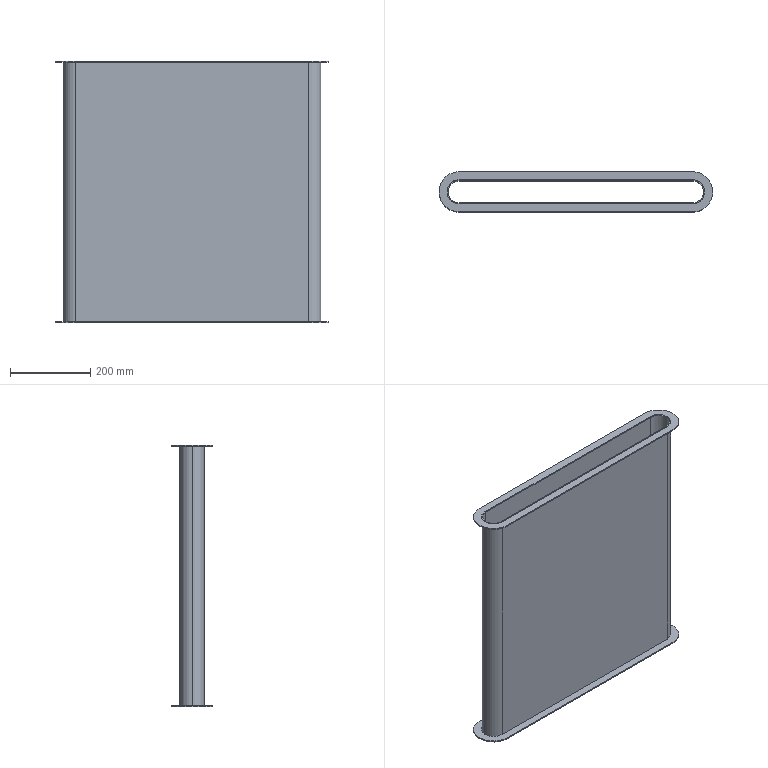Part | SolidWorks | features Extrusion 1, ICE 1, MirrorSolid 1 | 3 solids | 36 faces | box 680 x 100 x 650 mm | volume 2347902 mm3 | cylinder 18 | plane 18 | commonest cylinder face diameters 60 x9 100 x6 55 x3
STEP:
#1=CARTESIAN_POINT('',(0.,27.5,325.));
#2=VERTEX_POINT('',#1);
#3=CARTESIAN_POINT('',(-27.5,0.,325.));
#4=VERTEX_POINT('',#3);
#5=CARTESIAN_POINT('',(0.,0.,325.));
#6=DIRECTION('',(0.,0.,1.));
#7=DIRECTION('',(1.,0.,0.));
#8=AXIS2_PLACEMENT_3D('',#5,#6,#7);
#9=CIRCLE('',#8,27.5);
#10=EDGE_CURVE('',#2,#4,#9,.T.);
#11=ORIENTED_EDGE('',*,*,#10,.T.);
#12=CARTESIAN_POINT('',(-27.5,0.,-325.));
#13=VERTEX_POINT('',#12);
#14=CARTESIAN_POINT('',(-27.5,0.,325.));
#15=DIRECTION('',(0.,0.,-1.));
#16=VECTOR('',#15,1000.);
#17=LINE('',#14,#16);
#18=EDGE_CURVE('',#4,#13,#17,.T.);
#19=ORIENTED_EDGE('',*,*,#18,.T.);
#20=CARTESIAN_POINT('',(0.,27.5,-325.));
#21=VERTEX_POINT('',#20);
#22=CARTESIAN_POINT('',(0.,0.,-325.));
#23=DIRECTION('',(0.,0.,1.));
#24=DIRECTION('',(1.,0.,0.));
#25=AXIS2_PLACEMENT_3D('',#22,#23,#24);
#26=CIRCLE('',#25,27.5);
#27=EDGE_CURVE('',#21,#13,#26,.T.);
#28=ORIENTED_EDGE('',*,*,#27,.F.);
#29=CARTESIAN_POINT('',(0.,27.5,325.));
#30=DIRECTION('',(0.,0.,-1.));
#31=VECTOR('',#30,1000.);
#32=LINE('',#29,#31);
#33=EDGE_CURVE('',#2,#21,#32,.T.);
#34=ORIENTED_EDGE('',*,*,#33,.F.);
#35=EDGE_LOOP('',(#11,#19,#28,#34));
#36=FACE_OUTER_BOUND('',#35,.T.);
#37=CARTESIAN_POINT('',(0.,0.,325.));
#38=DIRECTION('',(0.,0.,-1.));
#39=DIRECTION('',(-1.,0.,0.));
#40=AXIS2_PLACEMENT_3D('',#37,#38,#39);
#41=CYLINDRICAL_SURFACE('',#40,27.5);
#42=ADVANCED_FACE('',(#36),#41,.F.);
#43=CARTESIAN_POINT('',(-30.,0.,325.));
#44=VERTEX_POINT('',#43);
#45=CARTESIAN_POINT('',(0.,-30.,325.));
#46=VERTEX_POINT('',#45);
#47=CARTESIAN_POINT('',(0.,0.,325.));
#48=DIRECTION('',(0.,0.,1.));
#49=DIRECTION('',(1.,0.,0.));
#50=AXIS2_PLACEMENT_3D('',#47,#48,#49);
#51=CIRCLE('',#50,30.);
#52=EDGE_CURVE('',#44,#46,#51,.T.);
#53=ORIENTED_EDGE('',*,*,#52,.F.);
#54=CARTESIAN_POINT('',(-30.,0.,-325.));
#55=VERTEX_POINT('',#54);
#56=CARTESIAN_POINT('',(-30.,0.,325.));
#57=DIRECTION('',(0.,0.,-1.));
#58=VECTOR('',#57,1000.);
#59=LINE('',#56,#58);
#60=EDGE_CURVE('',#44,#55,#59,.T.);
#61=ORIENTED_EDGE('',*,*,#60,.T.);
#62=CARTESIAN_POINT('',(0.,-30.,-325.));
#63=VERTEX_POINT('',#62);
#64=CARTESIAN_POINT('',(0.,0.,-325.));
#65=DIRECTION('',(0.,0.,1.));
#66=DIRECTION('',(1.,0.,0.));
#67=AXIS2_PLACEMENT_3D('',#64,#65,#66);
#68=CIRCLE('',#67,30.);
#69=EDGE_CURVE('',#55,#63,#68,.T.);
#70=ORIENTED_EDGE('',*,*,#69,.T.);
#71=CARTESIAN_POINT('',(0.,-30.,325.));
#72=DIRECTION('',(0.,0.,-1.));
#73=VECTOR('',#72,1000.);
#74=LINE('',#71,#73);
#75=EDGE_CURVE('',#46,#63,#74,.T.);
#76=ORIENTED_EDGE('',*,*,#75,.F.);
#77=EDGE_LOOP('',(#53,#61,#70,#76));
#78=FACE_OUTER_BOUND('',#77,.T.);
#79=CARTESIAN_POINT('',(0.,0.,325.));
#80=DIRECTION('',(0.,0.,-1.));
#81=DIRECTION('',(-1.,0.,0.));
#82=AXIS2_PLACEMENT_3D('',#79,#80,#81);
#83=CYLINDRICAL_SURFACE('',#82,30.);
#84=ADVANCED_FACE('',(#78),#83,.T.);
#85=CARTESIAN_POINT('',(0.,30.,325.));
#86=VERTEX_POINT('',#85);
#87=CARTESIAN_POINT('',(0.,0.,325.));
#88=DIRECTION('',(0.,0.,1.));
#89=DIRECTION('',(1.,0.,0.));
#90=AXIS2_PLACEMENT_3D('',#87,#88,#89);
#91=CIRCLE('',#90,30.);
#92=EDGE_CURVE('',#86,#44,#91,.T.);
#93=ORIENTED_EDGE('',*,*,#92,.T.);
#94=ORIENTED_EDGE('',*,*,#52,.T.);
#95=CARTESIAN_POINT('',(580.,-30.,325.));
#96=VERTEX_POINT('',#95);
#97=CARTESIAN_POINT('',(0.,-30.,325.));
#98=DIRECTION('',(1.,0.,0.));
#99=VECTOR('',#98,1000.);
#100=LINE('',#97,#99);
#101=EDGE_CURVE('',#46,#96,#100,.T.);
#102=ORIENTED_EDGE('',*,*,#101,.T.);
#103=CARTESIAN_POINT('',(580.,30.,325.));
#104=VERTEX_POINT('',#103);
#105=CARTESIAN_POINT('',(580.,0.,325.));
#106=DIRECTION('',(0.,0.,1.));
#107=DIRECTION('',(1.,0.,0.));
#108=AXIS2_PLACEMENT_3D('',#105,#106,#107);
#109=CIRCLE('',#108,30.);
#110=EDGE_CURVE('',#96,#104,#109,.T.);
#111=ORIENTED_EDGE('',*,*,#110,.T.);
#112=CARTESIAN_POINT('',(0.,30.,325.));
#113=DIRECTION('',(-1.,0.,0.));
#114=VECTOR('',#113,1000.);
#115=LINE('',#112,#114);
#116=EDGE_CURVE('',#104,#86,#115,.T.);
#117=ORIENTED_EDGE('',*,*,#116,.T.);
#118=EDGE_LOOP('',(#93,#94,#102,#111,#117));
#119=FACE_OUTER_BOUND('',#118,.T.);
#120=CARTESIAN_POINT('',(0.,-27.5,325.));
#121=VERTEX_POINT('',#120);
#122=CARTESIAN_POINT('',(580.,-27.5,325.));
#123=VERTEX_POINT('',#122);
#124=CARTESIAN_POINT('',(0.,-27.5,325.));
#125=DIRECTION('',(1.,0.,0.));
#126=VECTOR('',#125,1000.);
#127=LINE('',#124,#126);
#128=EDGE_CURVE('',#121,#123,#127,.T.);
#129=ORIENTED_EDGE('',*,*,#128,.F.);
#130=CARTESIAN_POINT('',(0.,0.,325.));
#131=DIRECTION('',(0.,0.,1.));
#132=DIRECTION('',(1.,0.,0.));
#133=AXIS2_PLACEMENT_3D('',#130,#131,#132);
#134=CIRCLE('',#133,27.5);
#135=EDGE_CURVE('',#4,#121,#134,.T.);
#136=ORIENTED_EDGE('',*,*,#135,.F.);
#137=ORIENTED_EDGE('',*,*,#10,.F.);
#138=CARTESIAN_POINT('',(580.,27.5,325.));
#139=VERTEX_POINT('',#138);
#140=CARTESIAN_POINT('',(0.,27.5,325.));
#141=DIRECTION('',(-1.,0.,0.));
#142=VECTOR('',#141,1000.);
#143=LINE('',#140,#142);
#144=EDGE_CURVE('',#139,#2,#143,.T.);
#145=ORIENTED_EDGE('',*,*,#144,.F.);
#146=CARTESIAN_POINT('',(580.,0.,325.));
#147=DIRECTION('',(0.,0.,1.));
#148=DIRECTION('',(1.,0.,0.));
#149=AXIS2_PLACEMENT_3D('',#146,#147,#148);
#150=CIRCLE('',#149,27.5);
#151=EDGE_CURVE('',#123,#139,#150,.T.);
#152=ORIENTED_EDGE('',*,*,#151,.F.);
#153=EDGE_LOOP('',(#129,#136,#137,#145,#152));
#154=FACE_BOUND('',#153,.T.);
#155=CARTESIAN_POINT('',(0.,0.,325.));
#156=DIRECTION('',(0.,0.,1.));
#157=DIRECTION('',(1.,0.,0.));
#158=AXIS2_PLACEMENT_3D('',#155,#156,#157);
#159=PLANE('',#158);
#160=ADVANCED_FACE('',(#119,#154),#159,.T.);
#161=CARTESIAN_POINT('',(0.,30.,-325.));
#162=VERTEX_POINT('',#161);
#163=CARTESIAN_POINT('',(0.,0.,-325.));
#164=DIRECTION('',(0.,0.,1.));
#165=DIRECTION('',(1.,0.,0.));
#166=AXIS2_PLACEMENT_3D('',#163,#164,#165);
#167=CIRCLE('',#166,30.);
#168=EDGE_CURVE('',#162,#55,#167,.T.);
#169=ORIENTED_EDGE('',*,*,#168,.F.);
#170=CARTESIAN_POINT('',(580.,30.,-325.));
#171=VERTEX_POINT('',#170);
#172=CARTESIAN_POINT('',(0.,30.,-325.));
#173=DIRECTION('',(-1.,0.,0.));
#174=VECTOR('',#173,1000.);
#175=LINE('',#172,#174);
#176=EDGE_CURVE('',#171,#162,#175,.T.);
#177=ORIENTED_EDGE('',*,*,#176,.F.);
#178=CARTESIAN_POINT('',(580.,-30.,-325.));
#179=VERTEX_POINT('',#178);
#180=CARTESIAN_POINT('',(580.,0.,-325.));
#181=DIRECTION('',(0.,0.,1.));
#182=DIRECTION('',(1.,0.,0.));
#183=AXIS2_PLACEMENT_3D('',#180,#181,#182);
#184=CIRCLE('',#183,30.);
#185=EDGE_CURVE('',#179,#171,#184,.T.);
#186=ORIENTED_EDGE('',*,*,#185,.F.);
#187=CARTESIAN_POINT('',(0.,-30.,-325.));
#188=DIRECTION('',(1.,0.,0.));
#189=VECTOR('',#188,1000.);
#190=LINE('',#187,#189);
#191=EDGE_CURVE('',#63,#179,#190,.T.);
#192=ORIENTED_EDGE('',*,*,#191,.F.);
#193=ORIENTED_EDGE('',*,*,#69,.F.);
#194=EDGE_LOOP('',(#169,#177,#186,#192,#193));
#195=FACE_OUTER_BOUND('',#194,.T.);
#196=ORIENTED_EDGE('',*,*,#27,.T.);
#197=CARTESIAN_POINT('',(0.,-27.5,-325.));
#198=VERTEX_POINT('',#197);
#199=CARTESIAN_POINT('',(0.,0.,-325.));
#200=DIRECTION('',(0.,0.,1.));
#201=DIRECTION('',(1.,0.,0.));
#202=AXIS2_PLACEMENT_3D('',#199,#200,#201);
#203=CIRCLE('',#202,27.5);
#204=EDGE_CURVE('',#13,#198,#203,.T.);
#205=ORIENTED_EDGE('',*,*,#204,.T.);
#206=CARTESIAN_POINT('',(580.,-27.5,-325.));
#207=VERTEX_POINT('',#206);
#208=CARTESIAN_POINT('',(0.,-27.5,-325.));
#209=DIRECTION('',(1.,0.,0.));
#210=VECTOR('',#209,1000.);
#211=LINE('',#208,#210);
#212=EDGE_CURVE('',#198,#207,#211,.T.);
#213=ORIENTED_EDGE('',*,*,#212,.T.);
#214=CARTESIAN_POINT('',(580.,27.5,-325.));
#215=VERTEX_POINT('',#214);
#216=CARTESIAN_POINT('',(580.,0.,-325.));
#217=DIRECTION('',(0.,0.,1.));
#218=DIRECTION('',(1.,0.,0.));
#219=AXIS2_PLACEMENT_3D('',#216,#217,#218);
#220=CIRCLE('',#219,27.5);
#221=EDGE_CURVE('',#207,#215,#220,.T.);
#222=ORIENTED_EDGE('',*,*,#221,.T.);
#223=CARTESIAN_POINT('',(0.,27.5,-325.));
#224=DIRECTION('',(-1.,0.,0.));
#225=VECTOR('',#224,1000.);
#226=LINE('',#223,#225);
#227=EDGE_CURVE('',#215,#21,#226,.T.);
#228=ORIENTED_EDGE('',*,*,#227,.T.);
#229=EDGE_LOOP('',(#196,#205,#213,#222,#228));
#230=FACE_BOUND('',#229,.T.);
#231=CARTESIAN_POINT('',(0.,0.,-325.));
#232=DIRECTION('',(0.,0.,1.));
#233=DIRECTION('',(1.,0.,0.));
#234=AXIS2_PLACEMENT_3D('',#231,#232,#233);
#235=PLANE('',#234);
#236=ADVANCED_FACE('',(#195,#230),#235,.F.);
#237=ORIENTED_EDGE('',*,*,#60,.F.);
#238=ORIENTED_EDGE('',*,*,#92,.F.);
#239=CARTESIAN_POINT('',(0.,30.,325.));
#240=DIRECTION('',(0.,0.,-1.));
#241=VECTOR('',#240,1000.);
#242=LINE('',#239,#241);
#243=EDGE_CURVE('',#86,#162,#242,.T.);
#244=ORIENTED_EDGE('',*,*,#243,.T.);
#245=ORIENTED_EDGE('',*,*,#168,.T.);
#246=EDGE_LOOP('',(#237,#238,#244,#245));
#247=FACE_OUTER_BOUND('',#246,.T.);
#248=CARTESIAN_POINT('',(0.,0.,325.));
#249=DIRECTION('',(0.,0.,-1.));
#250=DIRECTION('',(-1.,0.,0.));
#251=AXIS2_PLACEMENT_3D('',#248,#249,#250);
#252=CYLINDRICAL_SURFACE('',#251,30.);
#253=ADVANCED_FACE('',(#247),#252,.T.);
#254=ORIENTED_EDGE('',*,*,#191,.T.);
#255=CARTESIAN_POINT('',(580.,-30.,325.));
#256=DIRECTION('',(0.,0.,-1.));
#257=VECTOR('',#256,1000.);
#258=LINE('',#255,#257);
#259=EDGE_CURVE('',#96,#179,#258,.T.);
#260=ORIENTED_EDGE('',*,*,#259,.F.);
#261=ORIENTED_EDGE('',*,*,#101,.F.);
#262=ORIENTED_EDGE('',*,*,#75,.T.);
#263=EDGE_LOOP('',(#254,#260,#261,#262));
#264=FACE_OUTER_BOUND('',#263,.T.);
#265=CARTESIAN_POINT('',(0.,-30.,325.));
#266=DIRECTION('',(0.,1.,0.));
#267=DIRECTION('',(0.,0.,1.));
#268=AXIS2_PLACEMENT_3D('',#265,#266,#267);
#269=PLANE('',#268);
#270=ADVANCED_FACE('',(#264),#269,.F.);
#271=ORIENTED_EDGE('',*,*,#185,.T.);
#272=CARTESIAN_POINT('',(580.,30.,325.));
#273=DIRECTION('',(0.,0.,-1.));
#274=VECTOR('',#273,1000.);
#275=LINE('',#272,#274);
#276=EDGE_CURVE('',#104,#171,#275,.T.);
#277=ORIENTED_EDGE('',*,*,#276,.F.);
#278=ORIENTED_EDGE('',*,*,#110,.F.);
#279=ORIENTED_EDGE('',*,*,#259,.T.);
#280=EDGE_LOOP('',(#271,#277,#278,#279));
#281=FACE_OUTER_BOUND('',#280,.T.);
#282=CARTESIAN_POINT('',(580.,0.,325.));
#283=DIRECTION('',(0.,0.,-1.));
#284=DIRECTION('',(-1.,0.,0.));
#285=AXIS2_PLACEMENT_3D('',#282,#283,#284);
#286=CYLINDRICAL_SURFACE('',#285,30.);
#287=ADVANCED_FACE('',(#281),#286,.T.);
#288=ORIENTED_EDGE('',*,*,#176,.T.);
#289=ORIENTED_EDGE('',*,*,#243,.F.);
#290=ORIENTED_EDGE('',*,*,#116,.F.);
#291=ORIENTED_EDGE('',*,*,#276,.T.);
#292=EDGE_LOOP('',(#288,#289,#290,#291));
#293=FACE_OUTER_BOUND('',#292,.T.);
#294=CARTESIAN_POINT('',(0.,30.,325.));
#295=DIRECTION('',(0.,-1.,0.));
#296=DIRECTION('',(0.,0.,-1.));
#297=AXIS2_PLACEMENT_3D('',#294,#295,#296);
#298=PLANE('',#297);
#299=ADVANCED_FACE('',(#293),#298,.F.);
#300=ORIENTED_EDGE('',*,*,#18,.F.);
#301=ORIENTED_EDGE('',*,*,#135,.T.);
#302=CARTESIAN_POINT('',(0.,-27.5,325.));
#303=DIRECTION('',(0.,0.,-1.));
#304=VECTOR('',#303,1000.);
#305=LINE('',#302,#304);
#306=EDGE_CURVE('',#121,#198,#305,.T.);
#307=ORIENTED_EDGE('',*,*,#306,.T.);
#308=ORIENTED_EDGE('',*,*,#204,.F.);
#309=EDGE_LOOP('',(#300,#301,#307,#308));
#310=FACE_OUTER_BOUND('',#309,.T.);
#311=CARTESIAN_POINT('',(0.,0.,325.));
#312=DIRECTION('',(0.,0.,-1.));
#313=DIRECTION('',(-1.,0.,0.));
#314=AXIS2_PLACEMENT_3D('',#311,#312,#313);
#315=CYLINDRICAL_SURFACE('',#314,27.5);
#316=ADVANCED_FACE('',(#310),#315,.F.);
#317=ORIENTED_EDGE('',*,*,#212,.F.);
#318=ORIENTED_EDGE('',*,*,#306,.F.);
#319=ORIENTED_EDGE('',*,*,#128,.T.);
#320=CARTESIAN_POINT('',(580.,-27.5,325.));
#321=DIRECTION('',(0.,0.,-1.));
#322=VECTOR('',#321,1000.);
#323=LINE('',#320,#322);
#324=EDGE_CURVE('',#123,#207,#323,.T.);
#325=ORIENTED_EDGE('',*,*,#324,.T.);
#326=EDGE_LOOP('',(#317,#318,#319,#325));
#327=FACE_OUTER_BOUND('',#326,.T.);
#328=CARTESIAN_POINT('',(0.,-27.5,325.));
#329=DIRECTION('',(0.,1.,0.));
#330=DIRECTION('',(0.,0.,1.));
#331=AXIS2_PLACEMENT_3D('',#328,#329,#330);
#332=PLANE('',#331);
#333=ADVANCED_FACE('',(#327),#332,.T.);
#334=ORIENTED_EDGE('',*,*,#221,.F.);
#335=ORIENTED_EDGE('',*,*,#324,.F.);
#336=ORIENTED_EDGE('',*,*,#151,.T.);
#337=CARTESIAN_POINT('',(580.,27.5,325.));
#338=DIRECTION('',(0.,0.,-1.));
#339=VECTOR('',#338,1000.);
#340=LINE('',#337,#339);
#341=EDGE_CURVE('',#139,#215,#340,.T.);
#342=ORIENTED_EDGE('',*,*,#341,.T.);
#343=EDGE_LOOP('',(#334,#335,#336,#342));
#344=FACE_OUTER_BOUND('',#343,.T.);
#345=CARTESIAN_POINT('',(580.,0.,325.));
#346=DIRECTION('',(0.,0.,-1.));
#347=DIRECTION('',(-1.,0.,0.));
#348=AXIS2_PLACEMENT_3D('',#345,#346,#347);
#349=CYLINDRICAL_SURFACE('',#348,27.5);
#350=ADVANCED_FACE('',(#344),#349,.F.);
#351=ORIENTED_EDGE('',*,*,#227,.F.);
#352=ORIENTED_EDGE('',*,*,#341,.F.);
#353=ORIENTED_EDGE('',*,*,#144,.T.);
#354=ORIENTED_EDGE('',*,*,#33,.T.);
#355=EDGE_LOOP('',(#351,#352,#353,#354));
#356=FACE_OUTER_BOUND('',#355,.T.);
#357=CARTESIAN_POINT('',(0.,27.5,325.));
#358=DIRECTION('',(0.,-1.,0.));
#359=DIRECTION('',(0.,0.,-1.));
#360=AXIS2_PLACEMENT_3D('',#357,#358,#359);
#361=PLANE('',#360);
#362=ADVANCED_FACE('',(#356),#361,.T.);
#363=CLOSED_SHELL('',(#42,#84,#160,#236,#253,#270,#287,#299,#316,#333,#350,#362));
#364=MANIFOLD_SOLID_BREP('',#363);
#365=CARTESIAN_POINT('',(610.,0.,322.));
#366=VERTEX_POINT('',#365);
#367=CARTESIAN_POINT('',(580.,30.,322.));
#368=VERTEX_POINT('',#367);
#369=CARTESIAN_POINT('',(580.,0.,322.));
#370=DIRECTION('',(0.,0.,1.));
#371=DIRECTION('',(1.,0.,0.));
#372=AXIS2_PLACEMENT_3D('',#369,#370,#371);
#373=CIRCLE('',#372,30.);
#374=EDGE_CURVE('',#366,#368,#373,.T.);
#375=ORIENTED_EDGE('',*,*,#374,.F.);
#376=CARTESIAN_POINT('',(610.,0.,325.));
#377=VERTEX_POINT('',#376);
#378=CARTESIAN_POINT('',(610.,0.,322.));
#379=DIRECTION('',(0.,0.,1.));
#380=VECTOR('',#379,1000.);
#381=LINE('',#378,#380);
#382=EDGE_CURVE('',#366,#377,#381,.T.);
#383=ORIENTED_EDGE('',*,*,#382,.T.);
#384=CARTESIAN_POINT('',(580.,30.,325.));
#385=VERTEX_POINT('',#384);
#386=CARTESIAN_POINT('',(580.,0.,325.));
#387=DIRECTION('',(0.,0.,1.));
#388=DIRECTION('',(1.,0.,0.));
#389=AXIS2_PLACEMENT_3D('',#386,#387,#388);
#390=CIRCLE('',#389,30.);
#391=EDGE_CURVE('',#377,#385,#390,.T.);
#392=ORIENTED_EDGE('',*,*,#391,.T.);
#393=CARTESIAN_POINT('',(580.,30.,322.));
#394=DIRECTION('',(0.,0.,1.));
#395=VECTOR('',#394,1000.);
#396=LINE('',#393,#395);
#397=EDGE_CURVE('',#368,#385,#396,.T.);
#398=ORIENTED_EDGE('',*,*,#397,.F.);
#399=EDGE_LOOP('',(#375,#383,#392,#398));
#400=FACE_OUTER_BOUND('',#399,.T.);
#401=CARTESIAN_POINT('',(580.,0.,322.));
#402=DIRECTION('',(0.,0.,1.));
#403=DIRECTION('',(1.,0.,0.));
#404=AXIS2_PLACEMENT_3D('',#401,#402,#403);
#405=CYLINDRICAL_SURFACE('',#404,30.);
#406=ADVANCED_FACE('',(#400),#405,.F.);
#407=CARTESIAN_POINT('',(580.,-50.,322.));
#408=VERTEX_POINT('',#407);
#409=CARTESIAN_POINT('',(630.,0.,322.));
#410=VERTEX_POINT('',#409);
#411=CARTESIAN_POINT('',(580.,0.,322.));
#412=DIRECTION('',(0.,0.,1.));
#413=DIRECTION('',(1.,0.,0.));
#414=AXIS2_PLACEMENT_3D('',#411,#412,#413);
#415=CIRCLE('',#414,50.);
#416=EDGE_CURVE('',#408,#410,#415,.T.);
#417=ORIENTED_EDGE('',*,*,#416,.T.);
#418=CARTESIAN_POINT('',(630.,0.,325.));
#419=VERTEX_POINT('',#418);
#420=CARTESIAN_POINT('',(630.,0.,322.));
#421=DIRECTION('',(0.,0.,1.));
#422=VECTOR('',#421,1000.);
#423=LINE('',#420,#422);
#424=EDGE_CURVE('',#410,#419,#423,.T.);
#425=ORIENTED_EDGE('',*,*,#424,.T.);
#426=CARTESIAN_POINT('',(580.,-50.,325.));
#427=VERTEX_POINT('',#426);
#428=CARTESIAN_POINT('',(580.,0.,325.));
#429=DIRECTION('',(0.,0.,1.));
#430=DIRECTION('',(1.,0.,0.));
#431=AXIS2_PLACEMENT_3D('',#428,#429,#430);
#432=CIRCLE('',#431,50.);
#433=EDGE_CURVE('',#427,#419,#432,.T.);
#434=ORIENTED_EDGE('',*,*,#433,.F.);
#435=CARTESIAN_POINT('',(580.,-50.,322.));
#436=DIRECTION('',(0.,0.,1.));
#437=VECTOR('',#436,1000.);
#438=LINE('',#435,#437);
#439=EDGE_CURVE('',#408,#427,#438,.T.);
#440=ORIENTED_EDGE('',*,*,#439,.F.);
#441=EDGE_LOOP('',(#417,#425,#434,#440));
#442=FACE_OUTER_BOUND('',#441,.T.);
#443=CARTESIAN_POINT('',(580.,0.,322.));
#444=DIRECTION('',(0.,0.,1.));
#445=DIRECTION('',(1.,0.,0.));
#446=AXIS2_PLACEMENT_3D('',#443,#444,#445);
#447=CYLINDRICAL_SURFACE('',#446,50.);
#448=ADVANCED_FACE('',(#442),#447,.T.);
#449=ORIENTED_EDGE('',*,*,#424,.F.);
#450=CARTESIAN_POINT('',(580.,50.,322.));
#451=VERTEX_POINT('',#450);
#452=CARTESIAN_POINT('',(580.,0.,322.));
#453=DIRECTION('',(0.,0.,1.));
#454=DIRECTION('',(1.,0.,0.));
#455=AXIS2_PLACEMENT_3D('',#452,#453,#454);
#456=CIRCLE('',#455,50.);
#457=EDGE_CURVE('',#410,#451,#456,.T.);
#458=ORIENTED_EDGE('',*,*,#457,.T.);
#459=CARTESIAN_POINT('',(580.,50.,325.));
#460=VERTEX_POINT('',#459);
#461=CARTESIAN_POINT('',(580.,50.,322.));
#462=DIRECTION('',(0.,0.,1.));
#463=VECTOR('',#462,1000.);
#464=LINE('',#461,#463);
#465=EDGE_CURVE('',#451,#460,#464,.T.);
#466=ORIENTED_EDGE('',*,*,#465,.T.);
#467=CARTESIAN_POINT('',(580.,0.,325.));
#468=DIRECTION('',(0.,0.,1.));
#469=DIRECTION('',(1.,0.,0.));
#470=AXIS2_PLACEMENT_3D('',#467,#468,#469);
#471=CIRCLE('',#470,50.);
#472=EDGE_CURVE('',#419,#460,#471,.T.);
#473=ORIENTED_EDGE('',*,*,#472,.F.);
#474=EDGE_LOOP('',(#449,#458,#466,#473));
#475=FACE_OUTER_BOUND('',#474,.T.);
#476=CARTESIAN_POINT('',(580.,0.,322.));
#477=DIRECTION('',(0.,0.,1.));
#478=DIRECTION('',(1.,0.,0.));
#479=AXIS2_PLACEMENT_3D('',#476,#477,#478);
#480=CYLINDRICAL_SURFACE('',#479,50.);
#481=ADVANCED_FACE('',(#475),#480,.T.);
#482=CARTESIAN_POINT('',(0.,-50.,325.));
#483=VERTEX_POINT('',#482);
#484=CARTESIAN_POINT('',(0.,-50.,325.));
#485=DIRECTION('',(1.,0.,0.));
#486=VECTOR('',#485,1000.);
#487=LINE('',#484,#486);
#488=EDGE_CURVE('',#483,#427,#487,.T.);
#489=ORIENTED_EDGE('',*,*,#488,.F.);
#490=CARTESIAN_POINT('',(0.,-50.,322.));
#491=VERTEX_POINT('',#490);
#492=CARTESIAN_POINT('',(0.,-50.,322.));
#493=DIRECTION('',(0.,0.,1.));
#494=VECTOR('',#493,1000.);
#495=LINE('',#492,#494);
#496=EDGE_CURVE('',#491,#483,#495,.T.);
#497=ORIENTED_EDGE('',*,*,#496,.F.);
#498=CARTESIAN_POINT('',(0.,-50.,322.));
#499=DIRECTION('',(1.,0.,0.));
#500=VECTOR('',#499,1000.);
#501=LINE('',#498,#500);
#502=EDGE_CURVE('',#491,#408,#501,.T.);
#503=ORIENTED_EDGE('',*,*,#502,.T.);
#504=ORIENTED_EDGE('',*,*,#439,.T.);
#505=EDGE_LOOP('',(#489,#497,#503,#504));
#506=FACE_OUTER_BOUND('',#505,.T.);
#507=CARTESIAN_POINT('',(0.,-50.,322.));
#508=DIRECTION('',(0.,-1.,0.));
#509=DIRECTION('',(1.,0.,0.));
#510=AXIS2_PLACEMENT_3D('',#507,#508,#509);
#511=PLANE('',#510);
#512=ADVANCED_FACE('',(#506),#511,.T.);
#513=CARTESIAN_POINT('',(0.,50.,325.));
#514=VERTEX_POINT('',#513);
#515=CARTESIAN_POINT('',(0.,0.,325.));
#516=DIRECTION('',(0.,0.,1.));
#517=DIRECTION('',(1.,0.,0.));
#518=AXIS2_PLACEMENT_3D('',#515,#516,#517);
#519=CIRCLE('',#518,50.);
#520=EDGE_CURVE('',#514,#483,#519,.T.);
#521=ORIENTED_EDGE('',*,*,#520,.F.);
#522=CARTESIAN_POINT('',(0.,50.,322.));
#523=VERTEX_POINT('',#522);
#524=CARTESIAN_POINT('',(0.,50.,322.));
#525=DIRECTION('',(0.,0.,1.));
#526=VECTOR('',#525,1000.);
#527=LINE('',#524,#526);
#528=EDGE_CURVE('',#523,#514,#527,.T.);
#529=ORIENTED_EDGE('',*,*,#528,.F.);
#530=CARTESIAN_POINT('',(0.,0.,322.));
#531=DIRECTION('',(0.,0.,1.));
#532=DIRECTION('',(1.,0.,0.));
#533=AXIS2_PLACEMENT_3D('',#530,#531,#532);
#534=CIRCLE('',#533,50.);
#535=EDGE_CURVE('',#523,#491,#534,.T.);
#536=ORIENTED_EDGE('',*,*,#535,.T.);
#537=ORIENTED_EDGE('',*,*,#496,.T.);
#538=EDGE_LOOP('',(#521,#529,#536,#537));
#539=FACE_OUTER_BOUND('',#538,.T.);
#540=CARTESIAN_POINT('',(0.,0.,322.));
#541=DIRECTION('',(0.,0.,1.));
#542=DIRECTION('',(1.,0.,0.));
#543=AXIS2_PLACEMENT_3D('',#540,#541,#542);
#544=CYLINDRICAL_SURFACE('',#543,50.);
#545=ADVANCED_FACE('',(#539),#544,.T.);
#546=CARTESIAN_POINT('',(580.,50.,325.));
#547=DIRECTION('',(-1.,0.,0.));
#548=VECTOR('',#547,1000.);
#549=LINE('',#546,#548);
#550=EDGE_CURVE('',#460,#514,#549,.T.);
#551=ORIENTED_EDGE('',*,*,#550,.F.);
#552=ORIENTED_EDGE('',*,*,#465,.F.);
#553=CARTESIAN_POINT('',(580.,50.,322.));
#554=DIRECTION('',(-1.,0.,0.));
#555=VECTOR('',#554,1000.);
#556=LINE('',#553,#555);
#557=EDGE_CURVE('',#451,#523,#556,.T.);
#558=ORIENTED_EDGE('',*,*,#557,.T.);
#559=ORIENTED_EDGE('',*,*,#528,.T.);
#560=EDGE_LOOP('',(#551,#552,#558,#559));
#561=FACE_OUTER_BOUND('',#560,.T.);
#562=CARTESIAN_POINT('',(580.,50.,322.));
#563=DIRECTION('',(0.,1.,0.));
#564=DIRECTION('',(-1.,0.,0.));
#565=AXIS2_PLACEMENT_3D('',#562,#563,#564);
#566=PLANE('',#565);
#567=ADVANCED_FACE('',(#561),#566,.T.);
#568=CARTESIAN_POINT('',(0.,30.,322.));
#569=VERTEX_POINT('',#568);
#570=CARTESIAN_POINT('',(580.,30.,322.));
#571=DIRECTION('',(-1.,0.,0.));
#572=VECTOR('',#571,1000.);
#573=LINE('',#570,#572);
#574=EDGE_CURVE('',#368,#569,#573,.T.);
#575=ORIENTED_EDGE('',*,*,#574,.T.);
#576=CARTESIAN_POINT('',(0.,-30.,322.));
#577=VERTEX_POINT('',#576);
#578=CARTESIAN_POINT('',(0.,0.,322.));
#579=DIRECTION('',(0.,0.,1.));
#580=DIRECTION('',(1.,0.,0.));
#581=AXIS2_PLACEMENT_3D('',#578,#579,#580);
#582=CIRCLE('',#581,30.);
#583=EDGE_CURVE('',#569,#577,#582,.T.);
#584=ORIENTED_EDGE('',*,*,#583,.T.);
#585=CARTESIAN_POINT('',(580.,-30.,322.));
#586=VERTEX_POINT('',#585);
#587=CARTESIAN_POINT('',(0.,-30.,322.));
#588=DIRECTION('',(1.,0.,0.));
#589=VECTOR('',#588,1000.);
#590=LINE('',#587,#589);
#591=EDGE_CURVE('',#577,#586,#590,.T.);
#592=ORIENTED_EDGE('',*,*,#591,.T.);
#593=CARTESIAN_POINT('',(580.,0.,322.));
#594=DIRECTION('',(0.,0.,1.));
#595=DIRECTION('',(1.,0.,0.));
#596=AXIS2_PLACEMENT_3D('',#593,#594,#595);
#597=CIRCLE('',#596,30.);
#598=EDGE_CURVE('',#586,#366,#597,.T.);
#599=ORIENTED_EDGE('',*,*,#598,.T.);
#600=ORIENTED_EDGE('',*,*,#374,.T.);
#601=EDGE_LOOP('',(#575,#584,#592,#599,#600));
#602=FACE_BOUND('',#601,.T.);
#603=ORIENTED_EDGE('',*,*,#416,.F.);
#604=ORIENTED_EDGE('',*,*,#502,.F.);
#605=ORIENTED_EDGE('',*,*,#535,.F.);
#606=ORIENTED_EDGE('',*,*,#557,.F.);
#607=ORIENTED_EDGE('',*,*,#457,.F.);
#608=EDGE_LOOP('',(#603,#604,#605,#606,#607));
#609=FACE_OUTER_BOUND('',#608,.T.);
#610=CARTESIAN_POINT('',(580.,0.,322.));
#611=DIRECTION('',(0.,0.,1.));
#612=DIRECTION('',(1.,0.,0.));
#613=AXIS2_PLACEMENT_3D('',#610,#611,#612);
#614=PLANE('',#613);
#615=ADVANCED_FACE('',(#602,#609),#614,.F.);
#616=CARTESIAN_POINT('',(0.,30.,325.));
#617=VERTEX_POINT('',#616);
#618=CARTESIAN_POINT('',(0.,-30.,325.));
#619=VERTEX_POINT('',#618);
#620=CARTESIAN_POINT('',(0.,0.,325.));
#621=DIRECTION('',(0.,0.,1.));
#622=DIRECTION('',(1.,0.,0.));
#623=AXIS2_PLACEMENT_3D('',#620,#621,#622);
#624=CIRCLE('',#623,30.);
#625=EDGE_CURVE('',#617,#619,#624,.T.);
#626=ORIENTED_EDGE('',*,*,#625,.F.);
#627=CARTESIAN_POINT('',(580.,30.,325.));
#628=DIRECTION('',(-1.,0.,0.));
#629=VECTOR('',#628,1000.);
#630=LINE('',#627,#629);
#631=EDGE_CURVE('',#385,#617,#630,.T.);
#632=ORIENTED_EDGE('',*,*,#631,.F.);
#633=ORIENTED_EDGE('',*,*,#391,.F.);
#634=CARTESIAN_POINT('',(580.,-30.,325.));
#635=VERTEX_POINT('',#634);
#636=CARTESIAN_POINT('',(580.,0.,325.));
#637=DIRECTION('',(0.,0.,1.));
#638=DIRECTION('',(1.,0.,0.));
#639=AXIS2_PLACEMENT_3D('',#636,#637,#638);
#640=CIRCLE('',#639,30.);
#641=EDGE_CURVE('',#635,#377,#640,.T.);
#642=ORIENTED_EDGE('',*,*,#641,.F.);
#643=CARTESIAN_POINT('',(0.,-30.,325.));
#644=DIRECTION('',(1.,0.,0.));
#645=VECTOR('',#644,1000.);
#646=LINE('',#643,#645);
#647=EDGE_CURVE('',#619,#635,#646,.T.);
#648=ORIENTED_EDGE('',*,*,#647,.F.);
#649=EDGE_LOOP('',(#626,#632,#633,#642,#648));
#650=FACE_BOUND('',#649,.T.);
#651=ORIENTED_EDGE('',*,*,#433,.T.);
#652=ORIENTED_EDGE('',*,*,#472,.T.);
#653=ORIENTED_EDGE('',*,*,#550,.T.);
#654=ORIENTED_EDGE('',*,*,#520,.T.);
#655=ORIENTED_EDGE('',*,*,#488,.T.);
#656=EDGE_LOOP('',(#651,#652,#653,#654,#655));
#657=FACE_OUTER_BOUND('',#656,.T.);
#658=CARTESIAN_POINT('',(580.,0.,325.));
#659=DIRECTION('',(0.,0.,1.));
#660=DIRECTION('',(1.,0.,0.));
#661=AXIS2_PLACEMENT_3D('',#658,#659,#660);
#662=PLANE('',#661);
#663=ADVANCED_FACE('',(#650,#657),#662,.T.);
#664=ORIENTED_EDGE('',*,*,#625,.T.);
#665=CARTESIAN_POINT('',(0.,-30.,322.));
#666=DIRECTION('',(0.,0.,1.));
#667=VECTOR('',#666,1000.);
#668=LINE('',#665,#667);
#669=EDGE_CURVE('',#577,#619,#668,.T.);
#670=ORIENTED_EDGE('',*,*,#669,.F.);
#671=ORIENTED_EDGE('',*,*,#583,.F.);
#672=CARTESIAN_POINT('',(0.,30.,322.));
#673=DIRECTION('',(0.,0.,1.));
#674=VECTOR('',#673,1000.);
#675=LINE('',#672,#674);
#676=EDGE_CURVE('',#569,#617,#675,.T.);
#677=ORIENTED_EDGE('',*,*,#676,.T.);
#678=EDGE_LOOP('',(#664,#670,#671,#677));
#679=FACE_OUTER_BOUND('',#678,.T.);
#680=CARTESIAN_POINT('',(0.,0.,322.));
#681=DIRECTION('',(0.,0.,1.));
#682=DIRECTION('',(1.,0.,0.));
#683=AXIS2_PLACEMENT_3D('',#680,#681,#682);
#684=CYLINDRICAL_SURFACE('',#683,30.);
#685=ADVANCED_FACE('',(#679),#684,.F.);
#686=ORIENTED_EDGE('',*,*,#631,.T.);
#687=ORIENTED_EDGE('',*,*,#676,.F.);
#688=ORIENTED_EDGE('',*,*,#574,.F.);
#689=ORIENTED_EDGE('',*,*,#397,.T.);
#690=EDGE_LOOP('',(#686,#687,#688,#689));
#691=FACE_OUTER_BOUND('',#690,.T.);
#692=CARTESIAN_POINT('',(580.,30.,322.));
#693=DIRECTION('',(0.,1.,0.));
#694=DIRECTION('',(0.,0.,1.));
#695=AXIS2_PLACEMENT_3D('',#692,#693,#694);
#696=PLANE('',#695);
#697=ADVANCED_FACE('',(#691),#696,.F.);
#698=ORIENTED_EDGE('',*,*,#382,.F.);
#699=ORIENTED_EDGE('',*,*,#598,.F.);
#700=CARTESIAN_POINT('',(580.,-30.,322.));
#701=DIRECTION('',(0.,0.,1.));
#702=VECTOR('',#701,1000.);
#703=LINE('',#700,#702);
#704=EDGE_CURVE('',#586,#635,#703,.T.);
#705=ORIENTED_EDGE('',*,*,#704,.T.);
#706=ORIENTED_EDGE('',*,*,#641,.T.);
#707=EDGE_LOOP('',(#698,#699,#705,#706));
#708=FACE_OUTER_BOUND('',#707,.T.);
#709=CARTESIAN_POINT('',(580.,0.,322.));
#710=DIRECTION('',(0.,0.,1.));
#711=DIRECTION('',(1.,0.,0.));
#712=AXIS2_PLACEMENT_3D('',#709,#710,#711);
#713=CYLINDRICAL_SURFACE('',#712,30.);
#714=ADVANCED_FACE('',(#708),#713,.F.);
#715=ORIENTED_EDGE('',*,*,#647,.T.);
#716=ORIENTED_EDGE('',*,*,#704,.F.);
#717=ORIENTED_EDGE('',*,*,#591,.F.);
#718=ORIENTED_EDGE('',*,*,#669,.T.);
#719=EDGE_LOOP('',(#715,#716,#717,#718));
#720=FACE_OUTER_BOUND('',#719,.T.);
#721=CARTESIAN_POINT('',(0.,-30.,322.));
#722=DIRECTION('',(0.,-1.,0.));
#723=DIRECTION('',(0.,0.,-1.));
#724=AXIS2_PLACEMENT_3D('',#721,#722,#723);
#725=PLANE('',#724);
#726=ADVANCED_FACE('',(#720),#725,.F.);
#727=CLOSED_SHELL('',(#406,#448,#481,#512,#545,#567,#615,#663,#685,#697,#714,#726));
#728=MANIFOLD_SOLID_BREP('',#727);
#729=CARTESIAN_POINT('',(580.,-30.,-322.));
#730=VERTEX_POINT('',#729);
#731=CARTESIAN_POINT('',(610.,0.,-322.));
#732=VERTEX_POINT('',#731);
#733=CARTESIAN_POINT('',(580.,0.,-322.));
#734=DIRECTION('',(0.,0.,1.));
#735=DIRECTION('',(1.,0.,0.));
#736=AXIS2_PLACEMENT_3D('',#733,#734,#735);
#737=CIRCLE('',#736,30.);
#738=EDGE_CURVE('',#730,#732,#737,.T.);
#739=ORIENTED_EDGE('',*,*,#738,.T.);
#740=CARTESIAN_POINT('',(610.,0.,-325.));
#741=VERTEX_POINT('',#740);
#742=CARTESIAN_POINT('',(610.,0.,-322.));
#743=DIRECTION('',(0.,0.,-1.));
#744=VECTOR('',#743,1000.);
#745=LINE('',#742,#744);
#746=EDGE_CURVE('',#732,#741,#745,.T.);
#747=ORIENTED_EDGE('',*,*,#746,.T.);
#748=CARTESIAN_POINT('',(580.,-30.,-325.));
#749=VERTEX_POINT('',#748);
#750=CARTESIAN_POINT('',(580.,0.,-325.));
#751=DIRECTION('',(0.,0.,1.));
#752=DIRECTION('',(1.,0.,0.));
#753=AXIS2_PLACEMENT_3D('',#750,#751,#752);
#754=CIRCLE('',#753,30.);
#755=EDGE_CURVE('',#749,#741,#754,.T.);
#756=ORIENTED_EDGE('',*,*,#755,.F.);
#757=CARTESIAN_POINT('',(580.,-30.,-322.));
#758=DIRECTION('',(0.,0.,-1.));
#759=VECTOR('',#758,1000.);
#760=LINE('',#757,#759);
#761=EDGE_CURVE('',#730,#749,#760,.T.);
#762=ORIENTED_EDGE('',*,*,#761,.F.);
#763=EDGE_LOOP('',(#739,#747,#756,#762));
#764=FACE_OUTER_BOUND('',#763,.T.);
#765=CARTESIAN_POINT('',(580.,0.,-322.));
#766=DIRECTION('',(0.,0.,-1.));
#767=DIRECTION('',(1.,0.,0.));
#768=AXIS2_PLACEMENT_3D('',#765,#766,#767);
#769=CYLINDRICAL_SURFACE('',#768,30.);
#770=ADVANCED_FACE('',(#764),#769,.F.);
#771=CARTESIAN_POINT('',(630.,0.,-322.));
#772=VERTEX_POINT('',#771);
#773=CARTESIAN_POINT('',(580.,50.,-322.));
#774=VERTEX_POINT('',#773);
#775=CARTESIAN_POINT('',(580.,0.,-322.));
#776=DIRECTION('',(0.,0.,1.));
#777=DIRECTION('',(1.,0.,0.));
#778=AXIS2_PLACEMENT_3D('',#775,#776,#777);
#779=CIRCLE('',#778,50.);
#780=EDGE_CURVE('',#772,#774,#779,.T.);
#781=ORIENTED_EDGE('',*,*,#780,.F.);
#782=CARTESIAN_POINT('',(630.,0.,-325.));
#783=VERTEX_POINT('',#782);
#784=CARTESIAN_POINT('',(630.,0.,-322.));
#785=DIRECTION('',(0.,0.,-1.));
#786=VECTOR('',#785,1000.);
#787=LINE('',#784,#786);
#788=EDGE_CURVE('',#772,#783,#787,.T.);
#789=ORIENTED_EDGE('',*,*,#788,.T.);
#790=CARTESIAN_POINT('',(580.,50.,-325.));
#791=VERTEX_POINT('',#790);
#792=CARTESIAN_POINT('',(580.,0.,-325.));
#793=DIRECTION('',(0.,0.,1.));
#794=DIRECTION('',(1.,0.,0.));
#795=AXIS2_PLACEMENT_3D('',#792,#793,#794);
#796=CIRCLE('',#795,50.);
#797=EDGE_CURVE('',#783,#791,#796,.T.);
#798=ORIENTED_EDGE('',*,*,#797,.T.);
#799=CARTESIAN_POINT('',(580.,50.,-322.));
#800=DIRECTION('',(0.,0.,-1.));
#801=VECTOR('',#800,1000.);
#802=LINE('',#799,#801);
#803=EDGE_CURVE('',#774,#791,#802,.T.);
#804=ORIENTED_EDGE('',*,*,#803,.F.);
#805=EDGE_LOOP('',(#781,#789,#798,#804));
#806=FACE_OUTER_BOUND('',#805,.T.);
#807=CARTESIAN_POINT('',(580.,0.,-322.));
#808=DIRECTION('',(0.,0.,-1.));
#809=DIRECTION('',(1.,0.,0.));
#810=AXIS2_PLACEMENT_3D('',#807,#808,#809);
#811=CYLINDRICAL_SURFACE('',#810,50.);
#812=ADVANCED_FACE('',(#806),#811,.T.);
#813=ORIENTED_EDGE('',*,*,#788,.F.);
#814=CARTESIAN_POINT('',(580.,-50.,-322.));
#815=VERTEX_POINT('',#814);
#816=CARTESIAN_POINT('',(580.,0.,-322.));
#817=DIRECTION('',(0.,0.,1.));
#818=DIRECTION('',(1.,0.,0.));
#819=AXIS2_PLACEMENT_3D('',#816,#817,#818);
#820=CIRCLE('',#819,50.);
#821=EDGE_CURVE('',#815,#772,#820,.T.);
#822=ORIENTED_EDGE('',*,*,#821,.F.);
#823=CARTESIAN_POINT('',(580.,-50.,-325.));
#824=VERTEX_POINT('',#823);
#825=CARTESIAN_POINT('',(580.,-50.,-322.));
#826=DIRECTION('',(0.,0.,-1.));
#827=VECTOR('',#826,1000.);
#828=LINE('',#825,#827);
#829=EDGE_CURVE('',#815,#824,#828,.T.);
#830=ORIENTED_EDGE('',*,*,#829,.T.);
#831=CARTESIAN_POINT('',(580.,0.,-325.));
#832=DIRECTION('',(0.,0.,1.));
#833=DIRECTION('',(1.,0.,0.));
#834=AXIS2_PLACEMENT_3D('',#831,#832,#833);
#835=CIRCLE('',#834,50.);
#836=EDGE_CURVE('',#824,#783,#835,.T.);
#837=ORIENTED_EDGE('',*,*,#836,.T.);
#838=EDGE_LOOP('',(#813,#822,#830,#837));
#839=FACE_OUTER_BOUND('',#838,.T.);
#840=CARTESIAN_POINT('',(580.,0.,-322.));
#841=DIRECTION('',(0.,0.,-1.));
#842=DIRECTION('',(1.,0.,0.));
#843=AXIS2_PLACEMENT_3D('',#840,#841,#842);
#844=CYLINDRICAL_SURFACE('',#843,50.);
#845=ADVANCED_FACE('',(#839),#844,.T.);
#846=CARTESIAN_POINT('',(0.,-50.,-325.));
#847=VERTEX_POINT('',#846);
#848=CARTESIAN_POINT('',(0.,-50.,-325.));
#849=DIRECTION('',(1.,0.,0.));
#850=VECTOR('',#849,1000.);
#851=LINE('',#848,#850);
#852=EDGE_CURVE('',#847,#824,#851,.T.);
#853=ORIENTED_EDGE('',*,*,#852,.T.);
#854=ORIENTED_EDGE('',*,*,#829,.F.);
#855=CARTESIAN_POINT('',(0.,-50.,-322.));
#856=VERTEX_POINT('',#855);
#857=CARTESIAN_POINT('',(0.,-50.,-322.));
#858=DIRECTION('',(1.,0.,0.));
#859=VECTOR('',#858,1000.);
#860=LINE('',#857,#859);
#861=EDGE_CURVE('',#856,#815,#860,.T.);
#862=ORIENTED_EDGE('',*,*,#861,.F.);
#863=CARTESIAN_POINT('',(0.,-50.,-322.));
#864=DIRECTION('',(0.,0.,-1.));
#865=VECTOR('',#864,1000.);
#866=LINE('',#863,#865);
#867=EDGE_CURVE('',#856,#847,#866,.T.);
#868=ORIENTED_EDGE('',*,*,#867,.T.);
#869=EDGE_LOOP('',(#853,#854,#862,#868));
#870=FACE_OUTER_BOUND('',#869,.T.);
#871=CARTESIAN_POINT('',(0.,-50.,-322.));
#872=DIRECTION('',(0.,-1.,0.));
#873=DIRECTION('',(1.,0.,0.));
#874=AXIS2_PLACEMENT_3D('',#871,#872,#873);
#875=PLANE('',#874);
#876=ADVANCED_FACE('',(#870),#875,.T.);
#877=CARTESIAN_POINT('',(0.,50.,-325.));
#878=VERTEX_POINT('',#877);
#879=CARTESIAN_POINT('',(0.,0.,-325.));
#880=DIRECTION('',(0.,0.,1.));
#881=DIRECTION('',(1.,0.,0.));
#882=AXIS2_PLACEMENT_3D('',#879,#880,#881);
#883=CIRCLE('',#882,50.);
#884=EDGE_CURVE('',#878,#847,#883,.T.);
#885=ORIENTED_EDGE('',*,*,#884,.T.);
#886=ORIENTED_EDGE('',*,*,#867,.F.);
#887=CARTESIAN_POINT('',(0.,50.,-322.));
#888=VERTEX_POINT('',#887);
#889=CARTESIAN_POINT('',(0.,0.,-322.));
#890=DIRECTION('',(0.,0.,1.));
#891=DIRECTION('',(1.,0.,0.));
#892=AXIS2_PLACEMENT_3D('',#889,#890,#891);
#893=CIRCLE('',#892,50.);
#894=EDGE_CURVE('',#888,#856,#893,.T.);
#895=ORIENTED_EDGE('',*,*,#894,.F.);
#896=CARTESIAN_POINT('',(0.,50.,-322.));
#897=DIRECTION('',(0.,0.,-1.));
#898=VECTOR('',#897,1000.);
#899=LINE('',#896,#898);
#900=EDGE_CURVE('',#888,#878,#899,.T.);
#901=ORIENTED_EDGE('',*,*,#900,.T.);
#902=EDGE_LOOP('',(#885,#886,#895,#901));
#903=FACE_OUTER_BOUND('',#902,.T.);
#904=CARTESIAN_POINT('',(0.,0.,-322.));
#905=DIRECTION('',(0.,0.,-1.));
#906=DIRECTION('',(1.,0.,0.));
#907=AXIS2_PLACEMENT_3D('',#904,#905,#906);
#908=CYLINDRICAL_SURFACE('',#907,50.);
#909=ADVANCED_FACE('',(#903),#908,.T.);
#910=CARTESIAN_POINT('',(580.,50.,-325.));
#911=DIRECTION('',(-1.,0.,0.));
#912=VECTOR('',#911,1000.);
#913=LINE('',#910,#912);
#914=EDGE_CURVE('',#791,#878,#913,.T.);
#915=ORIENTED_EDGE('',*,*,#914,.T.);
#916=ORIENTED_EDGE('',*,*,#900,.F.);
#917=CARTESIAN_POINT('',(580.,50.,-322.));
#918=DIRECTION('',(-1.,0.,0.));
#919=VECTOR('',#918,1000.);
#920=LINE('',#917,#919);
#921=EDGE_CURVE('',#774,#888,#920,.T.);
#922=ORIENTED_EDGE('',*,*,#921,.F.);
#923=ORIENTED_EDGE('',*,*,#803,.T.);
#924=EDGE_LOOP('',(#915,#916,#922,#923));
#925=FACE_OUTER_BOUND('',#924,.T.);
#926=CARTESIAN_POINT('',(580.,50.,-322.));
#927=DIRECTION('',(0.,1.,0.));
#928=DIRECTION('',(-1.,0.,0.));
#929=AXIS2_PLACEMENT_3D('',#926,#927,#928);
#930=PLANE('',#929);
#931=ADVANCED_FACE('',(#925),#930,.T.);
#932=CARTESIAN_POINT('',(580.,30.,-322.));
#933=VERTEX_POINT('',#932);
#934=CARTESIAN_POINT('',(0.,30.,-322.));
#935=VERTEX_POINT('',#934);
#936=CARTESIAN_POINT('',(580.,30.,-322.));
#937=DIRECTION('',(-1.,0.,0.));
#938=VECTOR('',#937,1000.);
#939=LINE('',#936,#938);
#940=EDGE_CURVE('',#933,#935,#939,.T.);
#941=ORIENTED_EDGE('',*,*,#940,.F.);
#942=CARTESIAN_POINT('',(580.,0.,-322.));
#943=DIRECTION('',(0.,0.,1.));
#944=DIRECTION('',(1.,0.,0.));
#945=AXIS2_PLACEMENT_3D('',#942,#943,#944);
#946=CIRCLE('',#945,30.);
#947=EDGE_CURVE('',#732,#933,#946,.T.);
#948=ORIENTED_EDGE('',*,*,#947,.F.);
#949=ORIENTED_EDGE('',*,*,#738,.F.);
#950=CARTESIAN_POINT('',(0.,-30.,-322.));
#951=VERTEX_POINT('',#950);
#952=CARTESIAN_POINT('',(0.,-30.,-322.));
#953=DIRECTION('',(1.,0.,0.));
#954=VECTOR('',#953,1000.);
#955=LINE('',#952,#954);
#956=EDGE_CURVE('',#951,#730,#955,.T.);
#957=ORIENTED_EDGE('',*,*,#956,.F.);
#958=CARTESIAN_POINT('',(0.,0.,-322.));
#959=DIRECTION('',(0.,0.,1.));
#960=DIRECTION('',(1.,0.,0.));
#961=AXIS2_PLACEMENT_3D('',#958,#959,#960);
#962=CIRCLE('',#961,30.);
#963=EDGE_CURVE('',#935,#951,#962,.T.);
#964=ORIENTED_EDGE('',*,*,#963,.F.);
#965=EDGE_LOOP('',(#941,#948,#949,#957,#964));
#966=FACE_BOUND('',#965,.T.);
#967=ORIENTED_EDGE('',*,*,#821,.T.);
#968=ORIENTED_EDGE('',*,*,#780,.T.);
#969=ORIENTED_EDGE('',*,*,#921,.T.);
#970=ORIENTED_EDGE('',*,*,#894,.T.);
#971=ORIENTED_EDGE('',*,*,#861,.T.);
#972=EDGE_LOOP('',(#967,#968,#969,#970,#971));
#973=FACE_OUTER_BOUND('',#972,.T.);
#974=CARTESIAN_POINT('',(580.,0.,-322.));
#975=DIRECTION('',(0.,0.,-1.));
#976=DIRECTION('',(1.,0.,0.));
#977=AXIS2_PLACEMENT_3D('',#974,#975,#976);
#978=PLANE('',#977);
#979=ADVANCED_FACE('',(#966,#973),#978,.F.);
#980=CARTESIAN_POINT('',(0.,30.,-325.));
#981=VERTEX_POINT('',#980);
#982=CARTESIAN_POINT('',(0.,-30.,-325.));
#983=VERTEX_POINT('',#982);
#984=CARTESIAN_POINT('',(0.,0.,-325.));
#985=DIRECTION('',(0.,0.,1.));
#986=DIRECTION('',(1.,0.,0.));
#987=AXIS2_PLACEMENT_3D('',#984,#985,#986);
#988=CIRCLE('',#987,30.);
#989=EDGE_CURVE('',#981,#983,#988,.T.);
#990=ORIENTED_EDGE('',*,*,#989,.T.);
#991=CARTESIAN_POINT('',(0.,-30.,-325.));
#992=DIRECTION('',(1.,0.,0.));
#993=VECTOR('',#992,1000.);
#994=LINE('',#991,#993);
#995=EDGE_CURVE('',#983,#749,#994,.T.);
#996=ORIENTED_EDGE('',*,*,#995,.T.);
#997=ORIENTED_EDGE('',*,*,#755,.T.);
#998=CARTESIAN_POINT('',(580.,30.,-325.));
#999=VERTEX_POINT('',#998);
#1000=CARTESIAN_POINT('',(580.,0.,-325.));
#1001=DIRECTION('',(0.,0.,1.));
#1002=DIRECTION('',(1.,0.,0.));
#1003=AXIS2_PLACEMENT_3D('',#1000,#1001,#1002);
#1004=CIRCLE('',#1003,30.);
#1005=EDGE_CURVE('',#741,#999,#1004,.T.);
#1006=ORIENTED_EDGE('',*,*,#1005,.T.);
#1007=CARTESIAN_POINT('',(580.,30.,-325.));
#1008=DIRECTION('',(-1.,0.,0.));
#1009=VECTOR('',#1008,1000.);
#1010=LINE('',#1007,#1009);
#1011=EDGE_CURVE('',#999,#981,#1010,.T.);
#1012=ORIENTED_EDGE('',*,*,#1011,.T.);
#1013=EDGE_LOOP('',(#990,#996,#997,#1006,#1012));
#1014=FACE_BOUND('',#1013,.T.);
#1015=ORIENTED_EDGE('',*,*,#836,.F.);
#1016=ORIENTED_EDGE('',*,*,#852,.F.);
#1017=ORIENTED_EDGE('',*,*,#884,.F.);
#1018=ORIENTED_EDGE('',*,*,#914,.F.);
#1019=ORIENTED_EDGE('',*,*,#797,.F.);
#1020=EDGE_LOOP('',(#1015,#1016,#1017,#1018,#1019));
#1021=FACE_OUTER_BOUND('',#1020,.T.);
#1022=CARTESIAN_POINT('',(580.,0.,-325.));
#1023=DIRECTION('',(0.,0.,-1.));
#1024=DIRECTION('',(1.,0.,0.));
#1025=AXIS2_PLACEMENT_3D('',#1022,#1023,#1024);
#1026=PLANE('',#1025);
#1027=ADVANCED_FACE('',(#1014,#1021),#1026,.T.);
#1028=ORIENTED_EDGE('',*,*,#989,.F.);
#1029=CARTESIAN_POINT('',(0.,30.,-322.));
#1030=DIRECTION('',(0.,0.,-1.));
#1031=VECTOR('',#1030,1000.);
#1032=LINE('',#1029,#1031);
#1033=EDGE_CURVE('',#935,#981,#1032,.T.);
#1034=ORIENTED_EDGE('',*,*,#1033,.F.);
#1035=ORIENTED_EDGE('',*,*,#963,.T.);
#1036=CARTESIAN_POINT('',(0.,-30.,-322.));
#1037=DIRECTION('',(0.,0.,-1.));
#1038=VECTOR('',#1037,1000.);
#1039=LINE('',#1036,#1038);
#1040=EDGE_CURVE('',#951,#983,#1039,.T.);
#1041=ORIENTED_EDGE('',*,*,#1040,.T.);
#1042=EDGE_LOOP('',(#1028,#1034,#1035,#1041));
#1043=FACE_OUTER_BOUND('',#1042,.T.);
#1044=CARTESIAN_POINT('',(0.,0.,-322.));
#1045=DIRECTION('',(0.,0.,-1.));
#1046=DIRECTION('',(1.,0.,0.));
#1047=AXIS2_PLACEMENT_3D('',#1044,#1045,#1046);
#1048=CYLINDRICAL_SURFACE('',#1047,30.);
#1049=ADVANCED_FACE('',(#1043),#1048,.F.);
#1050=ORIENTED_EDGE('',*,*,#1011,.F.);
#1051=CARTESIAN_POINT('',(580.,30.,-322.));
#1052=DIRECTION('',(0.,0.,-1.));
#1053=VECTOR('',#1052,1000.);
#1054=LINE('',#1051,#1053);
#1055=EDGE_CURVE('',#933,#999,#1054,.T.);
#1056=ORIENTED_EDGE('',*,*,#1055,.F.);
#1057=ORIENTED_EDGE('',*,*,#940,.T.);
#1058=ORIENTED_EDGE('',*,*,#1033,.T.);
#1059=EDGE_LOOP('',(#1050,#1056,#1057,#1058));
#1060=FACE_OUTER_BOUND('',#1059,.T.);
#1061=CARTESIAN_POINT('',(580.,30.,-322.));
#1062=DIRECTION('',(0.,1.,0.));
#1063=DIRECTION('',(0.,0.,-1.));
#1064=AXIS2_PLACEMENT_3D('',#1061,#1062,#1063);
#1065=PLANE('',#1064);
#1066=ADVANCED_FACE('',(#1060),#1065,.F.);
#1067=ORIENTED_EDGE('',*,*,#746,.F.);
#1068=ORIENTED_EDGE('',*,*,#947,.T.);
#1069=ORIENTED_EDGE('',*,*,#1055,.T.);
#1070=ORIENTED_EDGE('',*,*,#1005,.F.);
#1071=EDGE_LOOP('',(#1067,#1068,#1069,#1070));
#1072=FACE_OUTER_BOUND('',#1071,.T.);
#1073=CARTESIAN_POINT('',(580.,0.,-322.));
#1074=DIRECTION('',(0.,0.,-1.));
#1075=DIRECTION('',(1.,0.,0.));
#1076=AXIS2_PLACEMENT_3D('',#1073,#1074,#1075);
#1077=CYLINDRICAL_SURFACE('',#1076,30.);
#1078=ADVANCED_FACE('',(#1072),#1077,.F.);
#1079=ORIENTED_EDGE('',*,*,#995,.F.);
#1080=ORIENTED_EDGE('',*,*,#1040,.F.);
#1081=ORIENTED_EDGE('',*,*,#956,.T.);
#1082=ORIENTED_EDGE('',*,*,#761,.T.);
#1083=EDGE_LOOP('',(#1079,#1080,#1081,#1082));
#1084=FACE_OUTER_BOUND('',#1083,.T.);
#1085=CARTESIAN_POINT('',(0.,-30.,-322.));
#1086=DIRECTION('',(0.,-1.,0.));
#1087=DIRECTION('',(0.,0.,1.));
#1088=AXIS2_PLACEMENT_3D('',#1085,#1086,#1087);
#1089=PLANE('',#1088);
#1090=ADVANCED_FACE('',(#1084),#1089,.F.);
#1091=CLOSED_SHELL('',(#770,#812,#845,#876,#909,#931,#979,#1027,#1049,#1066,#1078,#1090));
#1092=MANIFOLD_SOLID_BREP('',#1091);
#1093=CARTESIAN_POINT('',(0.,0.,0.));
#1094=DIRECTION('',(0.,0.,1.));
#1095=DIRECTION('',(1.,0.,0.));
#1096=AXIS2_PLACEMENT_3D('',#1093,#1094,#1095);
#1097=(LENGTH_UNIT()NAMED_UNIT(*)SI_UNIT(.MILLI.,.METRE.));
#1098=UNCERTAINTY_MEASURE_WITH_UNIT(LENGTH_MEASURE(0.00001),#1097,'','');
#1099=(NAMED_UNIT(*)PLANE_ANGLE_UNIT()SI_UNIT($,.RADIAN.));
#1100=(NAMED_UNIT(*)SI_UNIT($,.STERADIAN.)SOLID_ANGLE_UNIT());
#1101=(GEOMETRIC_REPRESENTATION_CONTEXT(3)GLOBAL_UNCERTAINTY_ASSIGNED_CONTEXT((#1098))GLOBAL_UNIT_ASSIGNED_CONTEXT((#1097,#1099,#1100))REPRESENTATION_CONTEXT('',''));
#1102=ADVANCED_BREP_SHAPE_REPRESENTATION('',(#364,#728,#1092,#1096),#1101);